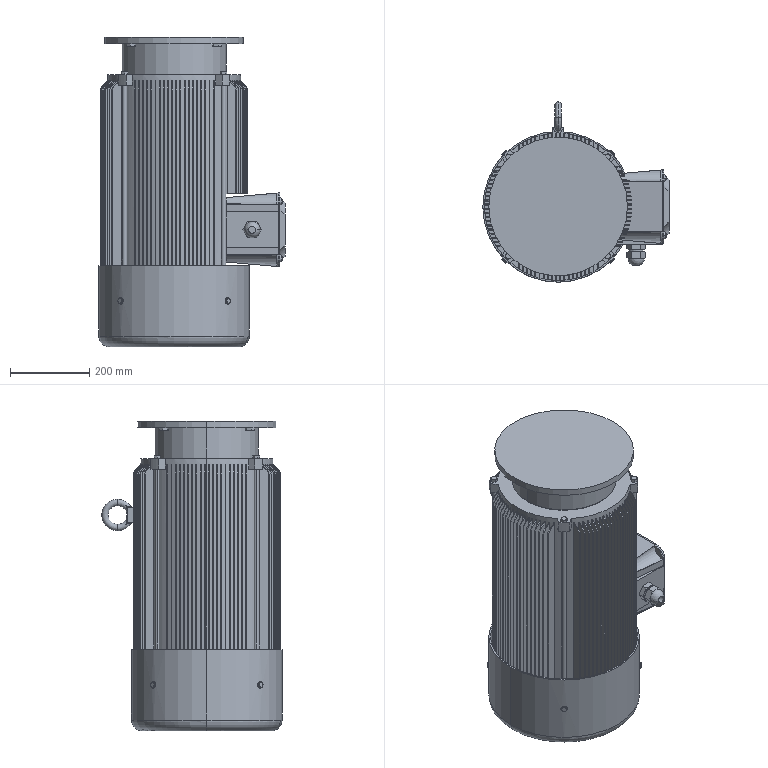Part | STEP file | 2 solids | 1037 faces | box 470 x 454.844 x 781 mm | volume 76496491 mm3 | plane 519 | cylinder 232 | cone 186 | torus 86 | other 8 | spline 4 | sphere 2 | commonest cylinder face diameters 370.952 x167 334.762 x23 10.857 x8 16.286 x8 36.19 x6 18.095 x4